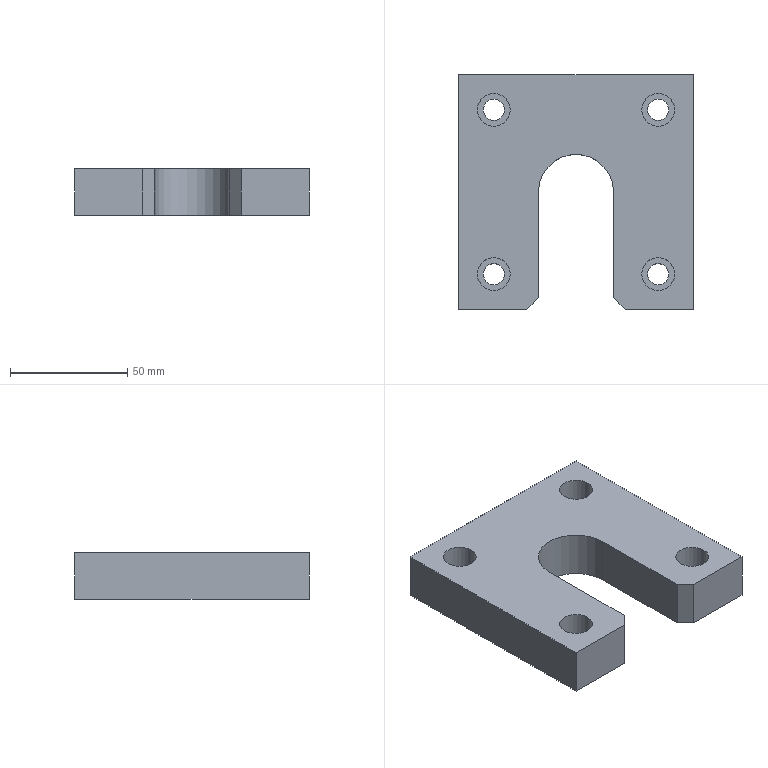Part | STEP file | 1 solid | 24 faces | box 100 x 100 x 20 mm | volume 150755 mm3 | plane 15 | cylinder 9 | commonest cylinder face diameters 9 x4 14 x4 32 x1
STEP:
#1=CARTESIAN_POINT('',(-434.,-292.5,-292.));
#2=VERTEX_POINT('',#1);
#3=CARTESIAN_POINT('',(-434.,-292.5,-272.));
#4=VERTEX_POINT('',#3);
#5=CARTESIAN_POINT('',(-434.,-292.5,-432.));
#6=DIRECTION('',(0.,0.,1.));
#7=VECTOR('',#6,1.);
#8=LINE('',#5,#7);
#9=EDGE_CURVE('',#2,#4,#8,.T.);
#10=ORIENTED_EDGE('',*,*,#9,.F.);
#11=CARTESIAN_POINT('',(-405.,-292.5,-292.));
#12=VERTEX_POINT('',#11);
#13=CARTESIAN_POINT('',(-455.,-292.5,-292.));
#14=DIRECTION('',(-1.,0.,0.));
#15=VECTOR('',#14,1.);
#16=LINE('',#13,#15);
#17=EDGE_CURVE('',#12,#2,#16,.T.);
#18=ORIENTED_EDGE('',*,*,#17,.F.);
#19=CARTESIAN_POINT('',(-405.,-292.5,-272.));
#20=VERTEX_POINT('',#19);
#21=CARTESIAN_POINT('',(-405.,-292.5,-292.));
#22=DIRECTION('',(0.,0.,1.));
#23=VECTOR('',#22,1.);
#24=LINE('',#21,#23);
#25=EDGE_CURVE('',#12,#20,#24,.T.);
#26=ORIENTED_EDGE('',*,*,#25,.T.);
#27=CARTESIAN_POINT('',(-455.,-292.5,-272.));
#28=DIRECTION('',(-1.,0.,0.));
#29=VECTOR('',#28,1.);
#30=LINE('',#27,#29);
#31=EDGE_CURVE('',#20,#4,#30,.T.);
#32=ORIENTED_EDGE('',*,*,#31,.T.);
#33=EDGE_LOOP('',(#10,#18,#26,#32));
#34=FACE_OUTER_BOUND('',#33,.T.);
#35=CARTESIAN_POINT('',(-455.,-292.5,-292.));
#36=DIRECTION('',(0.,1.,0.));
#37=DIRECTION('',(-1.,0.,0.));
#38=AXIS2_PLACEMENT_3D('',#35,#36,#37);
#39=PLANE('',#38);
#40=ADVANCED_FACE('',(#34),#39,.F.);
#41=CARTESIAN_POINT('',(-427.,-207.5,-272.));
#42=VERTEX_POINT('',#41);
#43=CARTESIAN_POINT('',(-420.,-207.5,-272.));
#44=DIRECTION('',(0.,0.,-1.));
#45=DIRECTION('',(-1.,0.,0.));
#46=AXIS2_PLACEMENT_3D('',#43,#44,#45);
#47=CIRCLE('',#46,7.);
#48=EDGE_CURVE('',#42,#42,#47,.T.);
#49=ORIENTED_EDGE('',*,*,#48,.T.);
#50=EDGE_LOOP('',(#49));
#51=FACE_BOUND('',#50,.T.);
#52=CARTESIAN_POINT('',(-483.,-207.5,-272.));
#53=VERTEX_POINT('',#52);
#54=CARTESIAN_POINT('',(-490.,-207.5,-272.));
#55=DIRECTION('',(0.,0.,1.));
#56=DIRECTION('',(1.,0.,0.));
#57=AXIS2_PLACEMENT_3D('',#54,#55,#56);
#58=CIRCLE('',#57,7.);
#59=EDGE_CURVE('',#53,#53,#58,.T.);
#60=ORIENTED_EDGE('',*,*,#59,.F.);
#61=EDGE_LOOP('',(#60));
#62=FACE_BOUND('',#61,.T.);
#63=CARTESIAN_POINT('',(-427.,-277.5,-272.));
#64=VERTEX_POINT('',#63);
#65=CARTESIAN_POINT('',(-420.,-277.5,-272.));
#66=DIRECTION('',(0.,0.,1.));
#67=DIRECTION('',(-1.,0.,0.));
#68=AXIS2_PLACEMENT_3D('',#65,#66,#67);
#69=CIRCLE('',#68,7.);
#70=EDGE_CURVE('',#64,#64,#69,.T.);
#71=ORIENTED_EDGE('',*,*,#70,.F.);
#72=EDGE_LOOP('',(#71));
#73=FACE_BOUND('',#72,.T.);
#74=CARTESIAN_POINT('',(-483.,-277.5,-272.));
#75=VERTEX_POINT('',#74);
#76=CARTESIAN_POINT('',(-490.,-277.5,-272.));
#77=DIRECTION('',(0.,0.,-1.));
#78=DIRECTION('',(1.,0.,0.));
#79=AXIS2_PLACEMENT_3D('',#76,#77,#78);
#80=CIRCLE('',#79,7.);
#81=EDGE_CURVE('',#75,#75,#80,.T.);
#82=ORIENTED_EDGE('',*,*,#81,.T.);
#83=EDGE_LOOP('',(#82));
#84=FACE_BOUND('',#83,.T.);
#85=CARTESIAN_POINT('',(-439.,-242.5,-272.));
#86=VERTEX_POINT('',#85);
#87=CARTESIAN_POINT('',(-439.,-287.5,-272.));
#88=VERTEX_POINT('',#87);
#89=CARTESIAN_POINT('',(-439.,-259.5,-272.));
#90=DIRECTION('',(0.,-1.,0.));
#91=VECTOR('',#90,1.);
#92=LINE('',#89,#91);
#93=EDGE_CURVE('',#86,#88,#92,.T.);
#94=ORIENTED_EDGE('',*,*,#93,.T.);
#95=CARTESIAN_POINT('',(-461.,-265.5,-272.));
#96=DIRECTION('',(0.7071,-0.7071,0.));
#97=VECTOR('',#96,1.);
#98=LINE('',#95,#97);
#99=EDGE_CURVE('',#88,#4,#98,.T.);
#100=ORIENTED_EDGE('',*,*,#99,.T.);
#101=ORIENTED_EDGE('',*,*,#31,.F.);
#102=CARTESIAN_POINT('',(-405.,-192.5,-272.));
#103=VERTEX_POINT('',#102);
#104=CARTESIAN_POINT('',(-405.,-259.5,-272.));
#105=DIRECTION('',(0.,-1.,0.));
#106=VECTOR('',#105,1.);
#107=LINE('',#104,#106);
#108=EDGE_CURVE('',#103,#20,#107,.T.);
#109=ORIENTED_EDGE('',*,*,#108,.F.);
#110=CARTESIAN_POINT('',(-505.,-192.5,-272.));
#111=VERTEX_POINT('',#110);
#112=CARTESIAN_POINT('',(-455.,-192.5,-272.));
#113=DIRECTION('',(1.,0.,0.));
#114=VECTOR('',#113,1.);
#115=LINE('',#112,#114);
#116=EDGE_CURVE('',#111,#103,#115,.T.);
#117=ORIENTED_EDGE('',*,*,#116,.F.);
#118=CARTESIAN_POINT('',(-505.,-292.5,-272.));
#119=VERTEX_POINT('',#118);
#120=CARTESIAN_POINT('',(-505.,-259.5,-272.));
#121=DIRECTION('',(0.,1.,0.));
#122=VECTOR('',#121,1.);
#123=LINE('',#120,#122);
#124=EDGE_CURVE('',#119,#111,#123,.T.);
#125=ORIENTED_EDGE('',*,*,#124,.F.);
#126=CARTESIAN_POINT('',(-476.,-292.5,-272.));
#127=VERTEX_POINT('',#126);
#128=CARTESIAN_POINT('',(-455.,-292.5,-272.));
#129=DIRECTION('',(-1.,0.,0.));
#130=VECTOR('',#129,1.);
#131=LINE('',#128,#130);
#132=EDGE_CURVE('',#127,#119,#131,.T.);
#133=ORIENTED_EDGE('',*,*,#132,.F.);
#134=CARTESIAN_POINT('',(-471.,-287.5,-272.));
#135=VERTEX_POINT('',#134);
#136=CARTESIAN_POINT('',(-449.,-265.5,-272.));
#137=DIRECTION('',(0.7071,0.7071,0.));
#138=VECTOR('',#137,1.);
#139=LINE('',#136,#138);
#140=EDGE_CURVE('',#127,#135,#139,.T.);
#141=ORIENTED_EDGE('',*,*,#140,.T.);
#142=CARTESIAN_POINT('',(-471.,-242.5,-272.));
#143=VERTEX_POINT('',#142);
#144=CARTESIAN_POINT('',(-471.,-259.5,-272.));
#145=DIRECTION('',(0.,1.,0.));
#146=VECTOR('',#145,1.);
#147=LINE('',#144,#146);
#148=EDGE_CURVE('',#135,#143,#147,.T.);
#149=ORIENTED_EDGE('',*,*,#148,.T.);
#150=CARTESIAN_POINT('',(-455.,-242.5,-272.));
#151=DIRECTION('',(0.,0.,-1.));
#152=DIRECTION('',(1.,0.,0.));
#153=AXIS2_PLACEMENT_3D('',#150,#151,#152);
#154=CIRCLE('',#153,16.);
#155=EDGE_CURVE('',#143,#86,#154,.T.);
#156=ORIENTED_EDGE('',*,*,#155,.T.);
#157=EDGE_LOOP('',(#94,#100,#101,#109,#117,#125,#133,#141,#149,#156));
#158=FACE_BOUND('',#157,.T.);
#159=CARTESIAN_POINT('',(-455.,-259.5,-272.));
#160=DIRECTION('',(0.,0.,1.));
#161=DIRECTION('',(1.,0.,0.));
#162=AXIS2_PLACEMENT_3D('',#159,#160,#161);
#163=PLANE('',#162);
#164=ADVANCED_FACE('',(#51,#62,#73,#84,#158),#163,.T.);
#165=CARTESIAN_POINT('',(-424.5,-207.5,-292.));
#166=VERTEX_POINT('',#165);
#167=CARTESIAN_POINT('',(-420.,-207.5,-292.));
#168=DIRECTION('',(0.,0.,1.));
#169=DIRECTION('',(-1.,0.,0.));
#170=AXIS2_PLACEMENT_3D('',#167,#168,#169);
#171=CIRCLE('',#170,4.5);
#172=EDGE_CURVE('',#166,#166,#171,.T.);
#173=ORIENTED_EDGE('',*,*,#172,.T.);
#174=EDGE_LOOP('',(#173));
#175=FACE_BOUND('',#174,.T.);
#176=CARTESIAN_POINT('',(-485.5,-207.5,-292.));
#177=VERTEX_POINT('',#176);
#178=CARTESIAN_POINT('',(-490.,-207.5,-292.));
#179=DIRECTION('',(0.,0.,-1.));
#180=DIRECTION('',(1.,0.,0.));
#181=AXIS2_PLACEMENT_3D('',#178,#179,#180);
#182=CIRCLE('',#181,4.5);
#183=EDGE_CURVE('',#177,#177,#182,.T.);
#184=ORIENTED_EDGE('',*,*,#183,.F.);
#185=EDGE_LOOP('',(#184));
#186=FACE_BOUND('',#185,.T.);
#187=CARTESIAN_POINT('',(-424.5,-277.5,-292.));
#188=VERTEX_POINT('',#187);
#189=CARTESIAN_POINT('',(-420.,-277.5,-292.));
#190=DIRECTION('',(0.,0.,-1.));
#191=DIRECTION('',(-1.,0.,0.));
#192=AXIS2_PLACEMENT_3D('',#189,#190,#191);
#193=CIRCLE('',#192,4.5);
#194=EDGE_CURVE('',#188,#188,#193,.T.);
#195=ORIENTED_EDGE('',*,*,#194,.F.);
#196=EDGE_LOOP('',(#195));
#197=FACE_BOUND('',#196,.T.);
#198=CARTESIAN_POINT('',(-485.5,-277.5,-292.));
#199=VERTEX_POINT('',#198);
#200=CARTESIAN_POINT('',(-490.,-277.5,-292.));
#201=DIRECTION('',(0.,0.,1.));
#202=DIRECTION('',(1.,0.,0.));
#203=AXIS2_PLACEMENT_3D('',#200,#201,#202);
#204=CIRCLE('',#203,4.5);
#205=EDGE_CURVE('',#199,#199,#204,.T.);
#206=ORIENTED_EDGE('',*,*,#205,.T.);
#207=EDGE_LOOP('',(#206));
#208=FACE_BOUND('',#207,.T.);
#209=CARTESIAN_POINT('',(-439.,-287.5,-292.));
#210=VERTEX_POINT('',#209);
#211=CARTESIAN_POINT('',(-461.,-265.5,-292.));
#212=DIRECTION('',(0.7071,-0.7071,0.));
#213=VECTOR('',#212,1.);
#214=LINE('',#211,#213);
#215=EDGE_CURVE('',#210,#2,#214,.T.);
#216=ORIENTED_EDGE('',*,*,#215,.F.);
#217=CARTESIAN_POINT('',(-439.,-242.5,-292.));
#218=VERTEX_POINT('',#217);
#219=CARTESIAN_POINT('',(-439.,-259.5,-292.));
#220=DIRECTION('',(0.,-1.,0.));
#221=VECTOR('',#220,1.);
#222=LINE('',#219,#221);
#223=EDGE_CURVE('',#218,#210,#222,.T.);
#224=ORIENTED_EDGE('',*,*,#223,.F.);
#225=CARTESIAN_POINT('',(-471.,-242.5,-292.));
#226=VERTEX_POINT('',#225);
#227=CARTESIAN_POINT('',(-455.,-242.5,-292.));
#228=DIRECTION('',(0.,0.,-1.));
#229=DIRECTION('',(1.,0.,0.));
#230=AXIS2_PLACEMENT_3D('',#227,#228,#229);
#231=CIRCLE('',#230,16.);
#232=EDGE_CURVE('',#226,#218,#231,.T.);
#233=ORIENTED_EDGE('',*,*,#232,.F.);
#234=CARTESIAN_POINT('',(-471.,-287.5,-292.));
#235=VERTEX_POINT('',#234);
#236=CARTESIAN_POINT('',(-471.,-259.5,-292.));
#237=DIRECTION('',(0.,1.,0.));
#238=VECTOR('',#237,1.);
#239=LINE('',#236,#238);
#240=EDGE_CURVE('',#235,#226,#239,.T.);
#241=ORIENTED_EDGE('',*,*,#240,.F.);
#242=CARTESIAN_POINT('',(-476.,-292.5,-292.));
#243=VERTEX_POINT('',#242);
#244=CARTESIAN_POINT('',(-449.,-265.5,-292.));
#245=DIRECTION('',(0.7071,0.7071,0.));
#246=VECTOR('',#245,1.);
#247=LINE('',#244,#246);
#248=EDGE_CURVE('',#243,#235,#247,.T.);
#249=ORIENTED_EDGE('',*,*,#248,.F.);
#250=CARTESIAN_POINT('',(-505.,-292.5,-292.));
#251=VERTEX_POINT('',#250);
#252=CARTESIAN_POINT('',(-455.,-292.5,-292.));
#253=DIRECTION('',(-1.,0.,0.));
#254=VECTOR('',#253,1.);
#255=LINE('',#252,#254);
#256=EDGE_CURVE('',#243,#251,#255,.T.);
#257=ORIENTED_EDGE('',*,*,#256,.T.);
#258=CARTESIAN_POINT('',(-505.,-192.5,-292.));
#259=VERTEX_POINT('',#258);
#260=CARTESIAN_POINT('',(-505.,-259.5,-292.));
#261=DIRECTION('',(0.,1.,0.));
#262=VECTOR('',#261,1.);
#263=LINE('',#260,#262);
#264=EDGE_CURVE('',#251,#259,#263,.T.);
#265=ORIENTED_EDGE('',*,*,#264,.T.);
#266=CARTESIAN_POINT('',(-405.,-192.5,-292.));
#267=VERTEX_POINT('',#266);
#268=CARTESIAN_POINT('',(-455.,-192.5,-292.));
#269=DIRECTION('',(1.,0.,0.));
#270=VECTOR('',#269,1.);
#271=LINE('',#268,#270);
#272=EDGE_CURVE('',#259,#267,#271,.T.);
#273=ORIENTED_EDGE('',*,*,#272,.T.);
#274=CARTESIAN_POINT('',(-405.,-259.5,-292.));
#275=DIRECTION('',(0.,-1.,0.));
#276=VECTOR('',#275,1.);
#277=LINE('',#274,#276);
#278=EDGE_CURVE('',#267,#12,#277,.T.);
#279=ORIENTED_EDGE('',*,*,#278,.T.);
#280=ORIENTED_EDGE('',*,*,#17,.T.);
#281=EDGE_LOOP('',(#216,#224,#233,#241,#249,#257,#265,#273,#279,#280));
#282=FACE_BOUND('',#281,.T.);
#283=CARTESIAN_POINT('',(-455.,-259.5,-292.));
#284=DIRECTION('',(0.,0.,1.));
#285=DIRECTION('',(1.,0.,0.));
#286=AXIS2_PLACEMENT_3D('',#283,#284,#285);
#287=PLANE('',#286);
#288=ADVANCED_FACE('',(#175,#186,#197,#208,#282),#287,.F.);
#289=ORIENTED_EDGE('',*,*,#25,.F.);
#290=ORIENTED_EDGE('',*,*,#278,.F.);
#291=CARTESIAN_POINT('',(-405.,-192.5,-292.));
#292=DIRECTION('',(0.,0.,1.));
#293=VECTOR('',#292,1.);
#294=LINE('',#291,#293);
#295=EDGE_CURVE('',#267,#103,#294,.T.);
#296=ORIENTED_EDGE('',*,*,#295,.T.);
#297=ORIENTED_EDGE('',*,*,#108,.T.);
#298=EDGE_LOOP('',(#289,#290,#296,#297));
#299=FACE_OUTER_BOUND('',#298,.T.);
#300=CARTESIAN_POINT('',(-405.,-259.5,-292.));
#301=DIRECTION('',(-1.,0.,0.));
#302=DIRECTION('',(0.,-1.,0.));
#303=AXIS2_PLACEMENT_3D('',#300,#301,#302);
#304=PLANE('',#303);
#305=ADVANCED_FACE('',(#299),#304,.F.);
#306=ORIENTED_EDGE('',*,*,#295,.F.);
#307=ORIENTED_EDGE('',*,*,#272,.F.);
#308=CARTESIAN_POINT('',(-505.,-192.5,-292.));
#309=DIRECTION('',(0.,0.,1.));
#310=VECTOR('',#309,1.);
#311=LINE('',#308,#310);
#312=EDGE_CURVE('',#259,#111,#311,.T.);
#313=ORIENTED_EDGE('',*,*,#312,.T.);
#314=ORIENTED_EDGE('',*,*,#116,.T.);
#315=EDGE_LOOP('',(#306,#307,#313,#314));
#316=FACE_OUTER_BOUND('',#315,.T.);
#317=CARTESIAN_POINT('',(-455.,-192.5,-292.));
#318=DIRECTION('',(0.,1.,0.));
#319=DIRECTION('',(-1.,0.,0.));
#320=AXIS2_PLACEMENT_3D('',#317,#318,#319);
#321=PLANE('',#320);
#322=ADVANCED_FACE('',(#316),#321,.T.);
#323=ORIENTED_EDGE('',*,*,#312,.F.);
#324=ORIENTED_EDGE('',*,*,#264,.F.);
#325=CARTESIAN_POINT('',(-505.,-292.5,-292.));
#326=DIRECTION('',(0.,0.,1.));
#327=VECTOR('',#326,1.);
#328=LINE('',#325,#327);
#329=EDGE_CURVE('',#251,#119,#328,.T.);
#330=ORIENTED_EDGE('',*,*,#329,.T.);
#331=ORIENTED_EDGE('',*,*,#124,.T.);
#332=EDGE_LOOP('',(#323,#324,#330,#331));
#333=FACE_OUTER_BOUND('',#332,.T.);
#334=CARTESIAN_POINT('',(-505.,-259.5,-292.));
#335=DIRECTION('',(1.,0.,0.));
#336=DIRECTION('',(0.,1.,0.));
#337=AXIS2_PLACEMENT_3D('',#334,#335,#336);
#338=PLANE('',#337);
#339=ADVANCED_FACE('',(#333),#338,.F.);
#340=CARTESIAN_POINT('',(-476.,-292.5,-432.));
#341=DIRECTION('',(0.,0.,-1.));
#342=VECTOR('',#341,1.);
#343=LINE('',#340,#342);
#344=EDGE_CURVE('',#127,#243,#343,.T.);
#345=ORIENTED_EDGE('',*,*,#344,.F.);
#346=ORIENTED_EDGE('',*,*,#132,.T.);
#347=ORIENTED_EDGE('',*,*,#329,.F.);
#348=ORIENTED_EDGE('',*,*,#256,.F.);
#349=EDGE_LOOP('',(#345,#346,#347,#348));
#350=FACE_OUTER_BOUND('',#349,.T.);
#351=CARTESIAN_POINT('',(-455.,-292.5,-292.));
#352=DIRECTION('',(0.,1.,0.));
#353=DIRECTION('',(-1.,0.,0.));
#354=AXIS2_PLACEMENT_3D('',#351,#352,#353);
#355=PLANE('',#354);
#356=ADVANCED_FACE('',(#350),#355,.F.);
#357=ORIENTED_EDGE('',*,*,#99,.F.);
#358=CARTESIAN_POINT('',(-439.,-287.5,-432.));
#359=DIRECTION('',(0.,0.,1.));
#360=VECTOR('',#359,1.);
#361=LINE('',#358,#360);
#362=EDGE_CURVE('',#210,#88,#361,.T.);
#363=ORIENTED_EDGE('',*,*,#362,.F.);
#364=ORIENTED_EDGE('',*,*,#215,.T.);
#365=ORIENTED_EDGE('',*,*,#9,.T.);
#366=EDGE_LOOP('',(#357,#363,#364,#365));
#367=FACE_OUTER_BOUND('',#366,.T.);
#368=CARTESIAN_POINT('',(-439.,-287.5,-432.));
#369=DIRECTION('',(-0.7071,-0.7071,0.));
#370=DIRECTION('',(0.7071,-0.7071,0.));
#371=AXIS2_PLACEMENT_3D('',#368,#369,#370);
#372=PLANE('',#371);
#373=ADVANCED_FACE('',(#367),#372,.T.);
#374=ORIENTED_EDGE('',*,*,#93,.F.);
#375=CARTESIAN_POINT('',(-439.,-242.5,-432.));
#376=DIRECTION('',(0.,0.,1.));
#377=VECTOR('',#376,1.);
#378=LINE('',#375,#377);
#379=EDGE_CURVE('',#218,#86,#378,.T.);
#380=ORIENTED_EDGE('',*,*,#379,.F.);
#381=ORIENTED_EDGE('',*,*,#223,.T.);
#382=ORIENTED_EDGE('',*,*,#362,.T.);
#383=EDGE_LOOP('',(#374,#380,#381,#382));
#384=FACE_OUTER_BOUND('',#383,.T.);
#385=CARTESIAN_POINT('',(-439.,-242.5,-432.));
#386=DIRECTION('',(-1.,0.,0.));
#387=DIRECTION('',(0.,0.,1.));
#388=AXIS2_PLACEMENT_3D('',#385,#386,#387);
#389=PLANE('',#388);
#390=ADVANCED_FACE('',(#384),#389,.T.);
#391=ORIENTED_EDGE('',*,*,#155,.F.);
#392=CARTESIAN_POINT('',(-471.,-242.5,-432.));
#393=DIRECTION('',(0.,0.,1.));
#394=VECTOR('',#393,1.);
#395=LINE('',#392,#394);
#396=EDGE_CURVE('',#226,#143,#395,.T.);
#397=ORIENTED_EDGE('',*,*,#396,.F.);
#398=ORIENTED_EDGE('',*,*,#232,.T.);
#399=ORIENTED_EDGE('',*,*,#379,.T.);
#400=EDGE_LOOP('',(#391,#397,#398,#399));
#401=FACE_OUTER_BOUND('',#400,.T.);
#402=CARTESIAN_POINT('',(-455.,-242.5,-432.));
#403=DIRECTION('',(0.,0.,1.));
#404=DIRECTION('',(1.,0.,0.));
#405=AXIS2_PLACEMENT_3D('',#402,#403,#404);
#406=CYLINDRICAL_SURFACE('',#405,16.);
#407=ADVANCED_FACE('',(#401),#406,.F.);
#408=ORIENTED_EDGE('',*,*,#148,.F.);
#409=CARTESIAN_POINT('',(-471.,-287.5,-432.));
#410=DIRECTION('',(0.,0.,1.));
#411=VECTOR('',#410,1.);
#412=LINE('',#409,#411);
#413=EDGE_CURVE('',#235,#135,#412,.T.);
#414=ORIENTED_EDGE('',*,*,#413,.F.);
#415=ORIENTED_EDGE('',*,*,#240,.T.);
#416=ORIENTED_EDGE('',*,*,#396,.T.);
#417=EDGE_LOOP('',(#408,#414,#415,#416));
#418=FACE_OUTER_BOUND('',#417,.T.);
#419=CARTESIAN_POINT('',(-471.,-287.5,-432.));
#420=DIRECTION('',(1.,0.,0.));
#421=DIRECTION('',(0.,0.,-1.));
#422=AXIS2_PLACEMENT_3D('',#419,#420,#421);
#423=PLANE('',#422);
#424=ADVANCED_FACE('',(#418),#423,.T.);
#425=ORIENTED_EDGE('',*,*,#140,.F.);
#426=ORIENTED_EDGE('',*,*,#344,.T.);
#427=ORIENTED_EDGE('',*,*,#248,.T.);
#428=ORIENTED_EDGE('',*,*,#413,.T.);
#429=EDGE_LOOP('',(#425,#426,#427,#428));
#430=FACE_OUTER_BOUND('',#429,.T.);
#431=CARTESIAN_POINT('',(-476.,-292.5,-432.));
#432=DIRECTION('',(0.7071,-0.7071,0.));
#433=DIRECTION('',(0.7071,0.7071,0.));
#434=AXIS2_PLACEMENT_3D('',#431,#432,#433);
#435=PLANE('',#434);
#436=ADVANCED_FACE('',(#430),#435,.T.);
#437=CARTESIAN_POINT('',(-494.5,-277.5,-282.));
#438=VERTEX_POINT('',#437);
#439=CARTESIAN_POINT('',(-490.,-277.5,-282.));
#440=DIRECTION('',(0.,0.,-1.));
#441=DIRECTION('',(-1.,0.,0.));
#442=AXIS2_PLACEMENT_3D('',#439,#440,#441);
#443=CIRCLE('',#442,4.5);
#444=EDGE_CURVE('',#438,#438,#443,.T.);
#445=ORIENTED_EDGE('',*,*,#444,.F.);
#446=EDGE_LOOP('',(#445));
#447=FACE_BOUND('',#446,.T.);
#448=ORIENTED_EDGE('',*,*,#205,.F.);
#449=EDGE_LOOP('',(#448));
#450=FACE_BOUND('',#449,.T.);
#451=CARTESIAN_POINT('',(-490.,-277.5,-292.));
#452=DIRECTION('',(0.,0.,1.));
#453=DIRECTION('',(1.,0.,0.));
#454=AXIS2_PLACEMENT_3D('',#451,#452,#453);
#455=CYLINDRICAL_SURFACE('',#454,4.5);
#456=ADVANCED_FACE('',(#447,#450),#455,.F.);
#457=ORIENTED_EDGE('',*,*,#444,.T.);
#458=EDGE_LOOP('',(#457));
#459=FACE_BOUND('',#458,.T.);
#460=CARTESIAN_POINT('',(-483.,-277.5,-282.));
#461=VERTEX_POINT('',#460);
#462=CARTESIAN_POINT('',(-490.,-277.5,-282.));
#463=DIRECTION('',(0.,0.,-1.));
#464=DIRECTION('',(1.,0.,0.));
#465=AXIS2_PLACEMENT_3D('',#462,#463,#464);
#466=CIRCLE('',#465,7.);
#467=EDGE_CURVE('',#461,#461,#466,.T.);
#468=ORIENTED_EDGE('',*,*,#467,.F.);
#469=EDGE_LOOP('',(#468));
#470=FACE_BOUND('',#469,.T.);
#471=CARTESIAN_POINT('',(-490.,-277.5,-282.));
#472=DIRECTION('',(0.,0.,-1.));
#473=DIRECTION('',(-1.,0.,0.));
#474=AXIS2_PLACEMENT_3D('',#471,#472,#473);
#475=PLANE('',#474);
#476=ADVANCED_FACE('',(#459,#470),#475,.F.);
#477=ORIENTED_EDGE('',*,*,#81,.F.);
#478=EDGE_LOOP('',(#477));
#479=FACE_BOUND('',#478,.T.);
#480=ORIENTED_EDGE('',*,*,#467,.T.);
#481=EDGE_LOOP('',(#480));
#482=FACE_BOUND('',#481,.T.);
#483=CARTESIAN_POINT('',(-490.,-277.5,-282.));
#484=DIRECTION('',(0.,0.,1.));
#485=DIRECTION('',(1.,0.,0.));
#486=AXIS2_PLACEMENT_3D('',#483,#484,#485);
#487=CYLINDRICAL_SURFACE('',#486,7.);
#488=ADVANCED_FACE('',(#479,#482),#487,.F.);
#489=CARTESIAN_POINT('',(-415.5,-277.5,-282.));
#490=VERTEX_POINT('',#489);
#491=CARTESIAN_POINT('',(-420.,-277.5,-282.));
#492=DIRECTION('',(0.,0.,1.));
#493=DIRECTION('',(1.,0.,0.));
#494=AXIS2_PLACEMENT_3D('',#491,#492,#493);
#495=CIRCLE('',#494,4.5);
#496=EDGE_CURVE('',#490,#490,#495,.T.);
#497=ORIENTED_EDGE('',*,*,#496,.T.);
#498=EDGE_LOOP('',(#497));
#499=FACE_BOUND('',#498,.T.);
#500=ORIENTED_EDGE('',*,*,#194,.T.);
#501=EDGE_LOOP('',(#500));
#502=FACE_BOUND('',#501,.T.);
#503=CARTESIAN_POINT('',(-420.,-277.5,-292.));
#504=DIRECTION('',(0.,0.,1.));
#505=DIRECTION('',(-1.,0.,0.));
#506=AXIS2_PLACEMENT_3D('',#503,#504,#505);
#507=CYLINDRICAL_SURFACE('',#506,4.5);
#508=ADVANCED_FACE('',(#499,#502),#507,.F.);
#509=ORIENTED_EDGE('',*,*,#496,.F.);
#510=EDGE_LOOP('',(#509));
#511=FACE_BOUND('',#510,.T.);
#512=CARTESIAN_POINT('',(-427.,-277.5,-282.));
#513=VERTEX_POINT('',#512);
#514=CARTESIAN_POINT('',(-420.,-277.5,-282.));
#515=DIRECTION('',(0.,0.,1.));
#516=DIRECTION('',(-1.,0.,0.));
#517=AXIS2_PLACEMENT_3D('',#514,#515,#516);
#518=CIRCLE('',#517,7.);
#519=EDGE_CURVE('',#513,#513,#518,.T.);
#520=ORIENTED_EDGE('',*,*,#519,.T.);
#521=EDGE_LOOP('',(#520));
#522=FACE_BOUND('',#521,.T.);
#523=CARTESIAN_POINT('',(-420.,-277.5,-282.));
#524=DIRECTION('',(0.,0.,-1.));
#525=DIRECTION('',(1.,0.,0.));
#526=AXIS2_PLACEMENT_3D('',#523,#524,#525);
#527=PLANE('',#526);
#528=ADVANCED_FACE('',(#511,#522),#527,.F.);
#529=ORIENTED_EDGE('',*,*,#70,.T.);
#530=EDGE_LOOP('',(#529));
#531=FACE_BOUND('',#530,.T.);
#532=ORIENTED_EDGE('',*,*,#519,.F.);
#533=EDGE_LOOP('',(#532));
#534=FACE_BOUND('',#533,.T.);
#535=CARTESIAN_POINT('',(-420.,-277.5,-282.));
#536=DIRECTION('',(0.,0.,1.));
#537=DIRECTION('',(-1.,0.,0.));
#538=AXIS2_PLACEMENT_3D('',#535,#536,#537);
#539=CYLINDRICAL_SURFACE('',#538,7.);
#540=ADVANCED_FACE('',(#531,#534),#539,.F.);
#541=CARTESIAN_POINT('',(-494.5,-207.5,-282.));
#542=VERTEX_POINT('',#541);
#543=CARTESIAN_POINT('',(-490.,-207.5,-282.));
#544=DIRECTION('',(0.,0.,1.));
#545=DIRECTION('',(-1.,0.,0.));
#546=AXIS2_PLACEMENT_3D('',#543,#544,#545);
#547=CIRCLE('',#546,4.5);
#548=EDGE_CURVE('',#542,#542,#547,.T.);
#549=ORIENTED_EDGE('',*,*,#548,.T.);
#550=EDGE_LOOP('',(#549));
#551=FACE_BOUND('',#550,.T.);
#552=ORIENTED_EDGE('',*,*,#183,.T.);
#553=EDGE_LOOP('',(#552));
#554=FACE_BOUND('',#553,.T.);
#555=CARTESIAN_POINT('',(-490.,-207.5,-292.));
#556=DIRECTION('',(0.,0.,1.));
#557=DIRECTION('',(1.,0.,0.));
#558=AXIS2_PLACEMENT_3D('',#555,#556,#557);
#559=CYLINDRICAL_SURFACE('',#558,4.5);
#560=ADVANCED_FACE('',(#551,#554),#559,.F.);
#561=ORIENTED_EDGE('',*,*,#548,.F.);
#562=EDGE_LOOP('',(#561));
#563=FACE_BOUND('',#562,.T.);
#564=CARTESIAN_POINT('',(-483.,-207.5,-282.));
#565=VERTEX_POINT('',#564);
#566=CARTESIAN_POINT('',(-490.,-207.5,-282.));
#567=DIRECTION('',(0.,0.,1.));
#568=DIRECTION('',(1.,0.,0.));
#569=AXIS2_PLACEMENT_3D('',#566,#567,#568);
#570=CIRCLE('',#569,7.);
#571=EDGE_CURVE('',#565,#565,#570,.T.);
#572=ORIENTED_EDGE('',*,*,#571,.T.);
#573=EDGE_LOOP('',(#572));
#574=FACE_BOUND('',#573,.T.);
#575=CARTESIAN_POINT('',(-490.,-207.5,-282.));
#576=DIRECTION('',(0.,0.,-1.));
#577=DIRECTION('',(-1.,0.,0.));
#578=AXIS2_PLACEMENT_3D('',#575,#576,#577);
#579=PLANE('',#578);
#580=ADVANCED_FACE('',(#563,#574),#579,.F.);
#581=ORIENTED_EDGE('',*,*,#59,.T.);
#582=EDGE_LOOP('',(#581));
#583=FACE_BOUND('',#582,.T.);
#584=ORIENTED_EDGE('',*,*,#571,.F.);
#585=EDGE_LOOP('',(#584));
#586=FACE_BOUND('',#585,.T.);
#587=CARTESIAN_POINT('',(-490.,-207.5,-282.));
#588=DIRECTION('',(0.,0.,1.));
#589=DIRECTION('',(1.,0.,0.));
#590=AXIS2_PLACEMENT_3D('',#587,#588,#589);
#591=CYLINDRICAL_SURFACE('',#590,7.);
#592=ADVANCED_FACE('',(#583,#586),#591,.F.);
#593=CARTESIAN_POINT('',(-415.5,-207.5,-282.));
#594=VERTEX_POINT('',#593);
#595=CARTESIAN_POINT('',(-420.,-207.5,-282.));
#596=DIRECTION('',(0.,0.,-1.));
#597=DIRECTION('',(1.,0.,0.));
#598=AXIS2_PLACEMENT_3D('',#595,#596,#597);
#599=CIRCLE('',#598,4.5);
#600=EDGE_CURVE('',#594,#594,#599,.T.);
#601=ORIENTED_EDGE('',*,*,#600,.F.);
#602=EDGE_LOOP('',(#601));
#603=FACE_BOUND('',#602,.T.);
#604=ORIENTED_EDGE('',*,*,#172,.F.);
#605=EDGE_LOOP('',(#604));
#606=FACE_BOUND('',#605,.T.);
#607=CARTESIAN_POINT('',(-420.,-207.5,-292.));
#608=DIRECTION('',(0.,0.,1.));
#609=DIRECTION('',(-1.,0.,0.));
#610=AXIS2_PLACEMENT_3D('',#607,#608,#609);
#611=CYLINDRICAL_SURFACE('',#610,4.5);
#612=ADVANCED_FACE('',(#603,#606),#611,.F.);
#613=ORIENTED_EDGE('',*,*,#600,.T.);
#614=EDGE_LOOP('',(#613));
#615=FACE_BOUND('',#614,.T.);
#616=CARTESIAN_POINT('',(-427.,-207.5,-282.));
#617=VERTEX_POINT('',#616);
#618=CARTESIAN_POINT('',(-420.,-207.5,-282.));
#619=DIRECTION('',(0.,0.,-1.));
#620=DIRECTION('',(-1.,0.,0.));
#621=AXIS2_PLACEMENT_3D('',#618,#619,#620);
#622=CIRCLE('',#621,7.);
#623=EDGE_CURVE('',#617,#617,#622,.T.);
#624=ORIENTED_EDGE('',*,*,#623,.F.);
#625=EDGE_LOOP('',(#624));
#626=FACE_BOUND('',#625,.T.);
#627=CARTESIAN_POINT('',(-420.,-207.5,-282.));
#628=DIRECTION('',(0.,0.,-1.));
#629=DIRECTION('',(1.,0.,0.));
#630=AXIS2_PLACEMENT_3D('',#627,#628,#629);
#631=PLANE('',#630);
#632=ADVANCED_FACE('',(#615,#626),#631,.F.);
#633=ORIENTED_EDGE('',*,*,#48,.F.);
#634=EDGE_LOOP('',(#633));
#635=FACE_BOUND('',#634,.T.);
#636=ORIENTED_EDGE('',*,*,#623,.T.);
#637=EDGE_LOOP('',(#636));
#638=FACE_BOUND('',#637,.T.);
#639=CARTESIAN_POINT('',(-420.,-207.5,-282.));
#640=DIRECTION('',(0.,0.,1.));
#641=DIRECTION('',(-1.,0.,0.));
#642=AXIS2_PLACEMENT_3D('',#639,#640,#641);
#643=CYLINDRICAL_SURFACE('',#642,7.);
#644=ADVANCED_FACE('',(#635,#638),#643,.F.);
#645=CLOSED_SHELL('',(#40,#164,#288,#305,#322,#339,#356,#373,#390,#407,#424,#436,#456,#476,#488,#508,#528,#540,#560,#580,#592,#612,#632,#644));
#646=MANIFOLD_SOLID_BREP('',#645);
#647=(LENGTH_UNIT()NAMED_UNIT(*)SI_UNIT(.MILLI.,.METRE.));
#648=UNCERTAINTY_MEASURE_WITH_UNIT(LENGTH_MEASURE(0.00002),#647,'','');
#649=(NAMED_UNIT(*)PLANE_ANGLE_UNIT()SI_UNIT($,.RADIAN.));
#650=PLANE_ANGLE_MEASURE_WITH_UNIT(PLANE_ANGLE_MEASURE(0.01745),#649);
#651=DIMENSIONAL_EXPONENTS(0.,0.,0.,0.,0.,0.,0.);
#652=(CONVERSION_BASED_UNIT('DEGREE',#650)NAMED_UNIT(#651)PLANE_ANGLE_UNIT());
#653=(NAMED_UNIT(*)SI_UNIT($,.STERADIAN.)SOLID_ANGLE_UNIT());
#654=(GEOMETRIC_REPRESENTATION_CONTEXT(3)GLOBAL_UNCERTAINTY_ASSIGNED_CONTEXT((#648))GLOBAL_UNIT_ASSIGNED_CONTEXT((#647,#652,#653))REPRESENTATION_CONTEXT('',''));
#655=ADVANCED_BREP_SHAPE_REPRESENTATION('',(#646),#654);